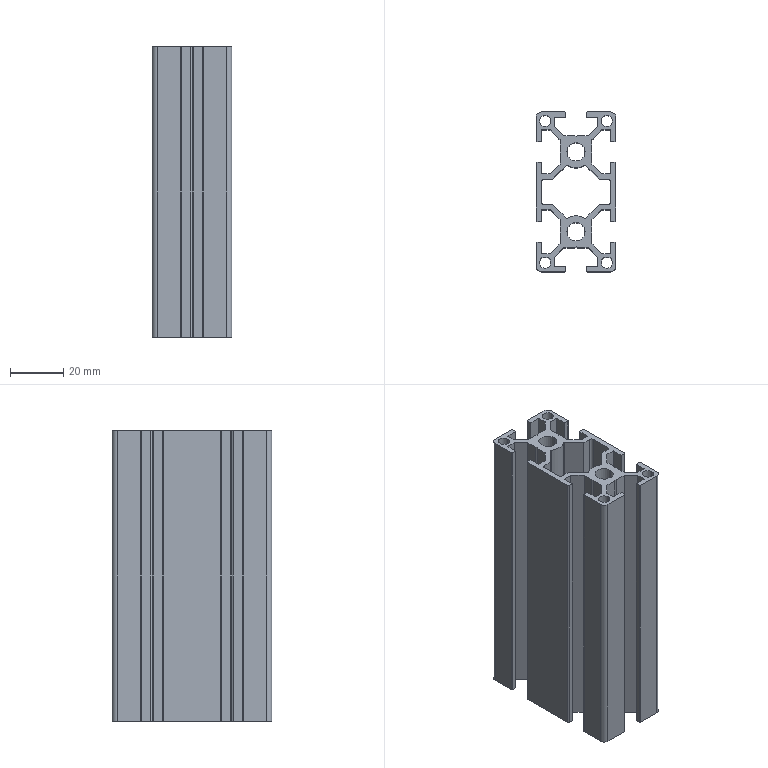Part | STEP file | Guide wheel mechanism revised.sldasm-Part-438 | 1 solid | 132 faces | box 30 x 60 x 109 mm | volume 64455 mm3 | plane 94 | cylinder 38 | commonest cylinder face diameters 0.6 x16 4.2 x8 2 x4 4 x4 6.8 x4 12 x2